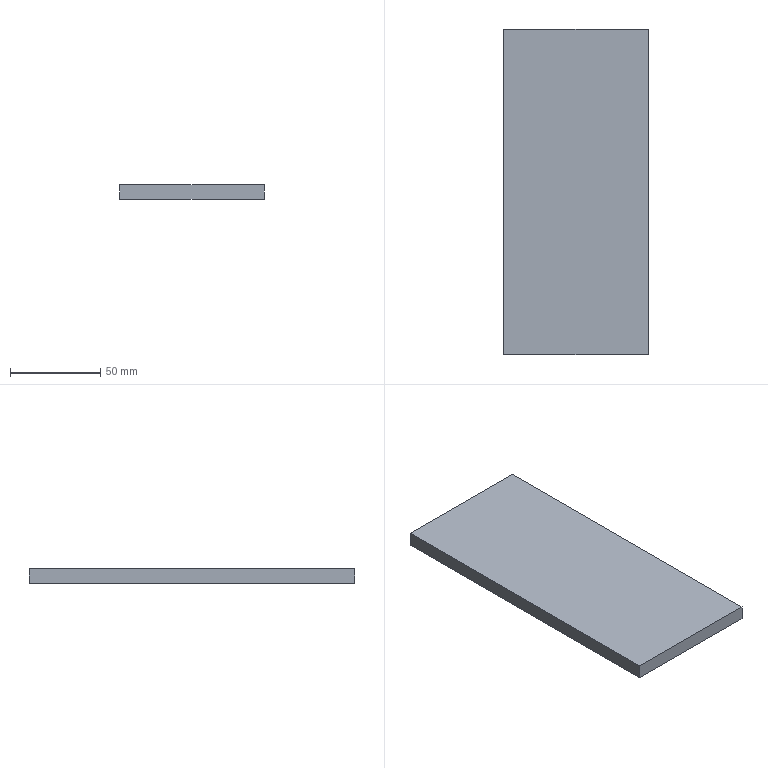Part | SolidWorks | features Extrusion 1 | 1 solid | 6 faces | box 80 x 180 x 8 mm | volume 115200 mm3 | plane 6
STEP:
#1=CARTESIAN_POINT('',(0.,180.,0.));
#2=VERTEX_POINT('',#1);
#3=CARTESIAN_POINT('',(0.,0.,0.));
#4=VERTEX_POINT('',#3);
#5=CARTESIAN_POINT('',(0.,180.,0.));
#6=DIRECTION('',(0.,-1.,0.));
#7=VECTOR('',#6,1000.);
#8=LINE('',#5,#7);
#9=EDGE_CURVE('',#2,#4,#8,.T.);
#10=ORIENTED_EDGE('',*,*,#9,.F.);
#11=CARTESIAN_POINT('',(0.,180.,-8.));
#12=VERTEX_POINT('',#11);
#13=CARTESIAN_POINT('',(0.,180.,-8.));
#14=DIRECTION('',(0.,0.,1.));
#15=VECTOR('',#14,1000.);
#16=LINE('',#13,#15);
#17=EDGE_CURVE('',#12,#2,#16,.T.);
#18=ORIENTED_EDGE('',*,*,#17,.F.);
#19=CARTESIAN_POINT('',(0.,0.,-8.));
#20=VERTEX_POINT('',#19);
#21=CARTESIAN_POINT('',(0.,180.,-8.));
#22=DIRECTION('',(0.,-1.,0.));
#23=VECTOR('',#22,1000.);
#24=LINE('',#21,#23);
#25=EDGE_CURVE('',#12,#20,#24,.T.);
#26=ORIENTED_EDGE('',*,*,#25,.T.);
#27=CARTESIAN_POINT('',(0.,0.,-8.));
#28=DIRECTION('',(0.,0.,1.));
#29=VECTOR('',#28,1000.);
#30=LINE('',#27,#29);
#31=EDGE_CURVE('',#20,#4,#30,.T.);
#32=ORIENTED_EDGE('',*,*,#31,.T.);
#33=EDGE_LOOP('',(#10,#18,#26,#32));
#34=FACE_OUTER_BOUND('',#33,.T.);
#35=CARTESIAN_POINT('',(0.,180.,-8.));
#36=DIRECTION('',(-1.,0.,0.));
#37=DIRECTION('',(0.,0.,1.));
#38=AXIS2_PLACEMENT_3D('',#35,#36,#37);
#39=PLANE('',#38);
#40=ADVANCED_FACE('',(#34),#39,.T.);
#41=CARTESIAN_POINT('',(80.,180.,0.));
#42=VERTEX_POINT('',#41);
#43=CARTESIAN_POINT('',(80.,180.,0.));
#44=DIRECTION('',(-1.,0.,0.));
#45=VECTOR('',#44,1000.);
#46=LINE('',#43,#45);
#47=EDGE_CURVE('',#42,#2,#46,.T.);
#48=ORIENTED_EDGE('',*,*,#47,.F.);
#49=CARTESIAN_POINT('',(80.,180.,-8.));
#50=VERTEX_POINT('',#49);
#51=CARTESIAN_POINT('',(80.,180.,-8.));
#52=DIRECTION('',(0.,0.,1.));
#53=VECTOR('',#52,1000.);
#54=LINE('',#51,#53);
#55=EDGE_CURVE('',#50,#42,#54,.T.);
#56=ORIENTED_EDGE('',*,*,#55,.F.);
#57=CARTESIAN_POINT('',(80.,180.,-8.));
#58=DIRECTION('',(-1.,0.,0.));
#59=VECTOR('',#58,1000.);
#60=LINE('',#57,#59);
#61=EDGE_CURVE('',#50,#12,#60,.T.);
#62=ORIENTED_EDGE('',*,*,#61,.T.);
#63=ORIENTED_EDGE('',*,*,#17,.T.);
#64=EDGE_LOOP('',(#48,#56,#62,#63));
#65=FACE_OUTER_BOUND('',#64,.T.);
#66=CARTESIAN_POINT('',(80.,180.,-8.));
#67=DIRECTION('',(0.,1.,0.));
#68=DIRECTION('',(0.,0.,1.));
#69=AXIS2_PLACEMENT_3D('',#66,#67,#68);
#70=PLANE('',#69);
#71=ADVANCED_FACE('',(#65),#70,.T.);
#72=CARTESIAN_POINT('',(80.,0.,0.));
#73=VERTEX_POINT('',#72);
#74=CARTESIAN_POINT('',(80.,0.,0.));
#75=DIRECTION('',(0.,1.,0.));
#76=VECTOR('',#75,1000.);
#77=LINE('',#74,#76);
#78=EDGE_CURVE('',#73,#42,#77,.T.);
#79=ORIENTED_EDGE('',*,*,#78,.F.);
#80=CARTESIAN_POINT('',(80.,0.,-8.));
#81=VERTEX_POINT('',#80);
#82=CARTESIAN_POINT('',(80.,0.,-8.));
#83=DIRECTION('',(0.,0.,1.));
#84=VECTOR('',#83,1000.);
#85=LINE('',#82,#84);
#86=EDGE_CURVE('',#81,#73,#85,.T.);
#87=ORIENTED_EDGE('',*,*,#86,.F.);
#88=CARTESIAN_POINT('',(80.,0.,-8.));
#89=DIRECTION('',(0.,1.,0.));
#90=VECTOR('',#89,1000.);
#91=LINE('',#88,#90);
#92=EDGE_CURVE('',#81,#50,#91,.T.);
#93=ORIENTED_EDGE('',*,*,#92,.T.);
#94=ORIENTED_EDGE('',*,*,#55,.T.);
#95=EDGE_LOOP('',(#79,#87,#93,#94));
#96=FACE_OUTER_BOUND('',#95,.T.);
#97=CARTESIAN_POINT('',(80.,0.,-8.));
#98=DIRECTION('',(1.,0.,0.));
#99=DIRECTION('',(0.,0.,-1.));
#100=AXIS2_PLACEMENT_3D('',#97,#98,#99);
#101=PLANE('',#100);
#102=ADVANCED_FACE('',(#96),#101,.T.);
#103=CARTESIAN_POINT('',(0.,0.,0.));
#104=DIRECTION('',(1.,0.,0.));
#105=VECTOR('',#104,1000.);
#106=LINE('',#103,#105);
#107=EDGE_CURVE('',#4,#73,#106,.T.);
#108=ORIENTED_EDGE('',*,*,#107,.F.);
#109=ORIENTED_EDGE('',*,*,#31,.F.);
#110=CARTESIAN_POINT('',(0.,0.,-8.));
#111=DIRECTION('',(1.,0.,0.));
#112=VECTOR('',#111,1000.);
#113=LINE('',#110,#112);
#114=EDGE_CURVE('',#20,#81,#113,.T.);
#115=ORIENTED_EDGE('',*,*,#114,.T.);
#116=ORIENTED_EDGE('',*,*,#86,.T.);
#117=EDGE_LOOP('',(#108,#109,#115,#116));
#118=FACE_OUTER_BOUND('',#117,.T.);
#119=CARTESIAN_POINT('',(0.,0.,-8.));
#120=DIRECTION('',(0.,-1.,0.));
#121=DIRECTION('',(0.,0.,-1.));
#122=AXIS2_PLACEMENT_3D('',#119,#120,#121);
#123=PLANE('',#122);
#124=ADVANCED_FACE('',(#118),#123,.T.);
#125=ORIENTED_EDGE('',*,*,#25,.F.);
#126=ORIENTED_EDGE('',*,*,#61,.F.);
#127=ORIENTED_EDGE('',*,*,#92,.F.);
#128=ORIENTED_EDGE('',*,*,#114,.F.);
#129=EDGE_LOOP('',(#125,#126,#127,#128));
#130=FACE_OUTER_BOUND('',#129,.T.);
#131=CARTESIAN_POINT('',(0.,0.,-8.));
#132=DIRECTION('',(0.,0.,1.));
#133=DIRECTION('',(1.,0.,0.));
#134=AXIS2_PLACEMENT_3D('',#131,#132,#133);
#135=PLANE('',#134);
#136=ADVANCED_FACE('',(#130),#135,.F.);
#137=ORIENTED_EDGE('',*,*,#9,.T.);
#138=ORIENTED_EDGE('',*,*,#107,.T.);
#139=ORIENTED_EDGE('',*,*,#78,.T.);
#140=ORIENTED_EDGE('',*,*,#47,.T.);
#141=EDGE_LOOP('',(#137,#138,#139,#140));
#142=FACE_OUTER_BOUND('',#141,.T.);
#143=CARTESIAN_POINT('',(0.,0.,0.));
#144=DIRECTION('',(0.,0.,1.));
#145=DIRECTION('',(1.,0.,0.));
#146=AXIS2_PLACEMENT_3D('',#143,#144,#145);
#147=PLANE('',#146);
#148=ADVANCED_FACE('',(#142),#147,.T.);
#149=CLOSED_SHELL('',(#40,#71,#102,#124,#136,#148));
#150=MANIFOLD_SOLID_BREP('',#149);
#151=CARTESIAN_POINT('',(0.,0.,0.));
#152=DIRECTION('',(0.,0.,1.));
#153=DIRECTION('',(1.,0.,0.));
#154=AXIS2_PLACEMENT_3D('',#151,#152,#153);
#155=(LENGTH_UNIT()NAMED_UNIT(*)SI_UNIT(.MILLI.,.METRE.));
#156=UNCERTAINTY_MEASURE_WITH_UNIT(LENGTH_MEASURE(0.00001),#155,'','');
#157=(NAMED_UNIT(*)PLANE_ANGLE_UNIT()SI_UNIT($,.RADIAN.));
#158=(NAMED_UNIT(*)SI_UNIT($,.STERADIAN.)SOLID_ANGLE_UNIT());
#159=(GEOMETRIC_REPRESENTATION_CONTEXT(3)GLOBAL_UNCERTAINTY_ASSIGNED_CONTEXT((#156))GLOBAL_UNIT_ASSIGNED_CONTEXT((#155,#157,#158))REPRESENTATION_CONTEXT('',''));
#160=ADVANCED_BREP_SHAPE_REPRESENTATION('',(#150,#154),#159);